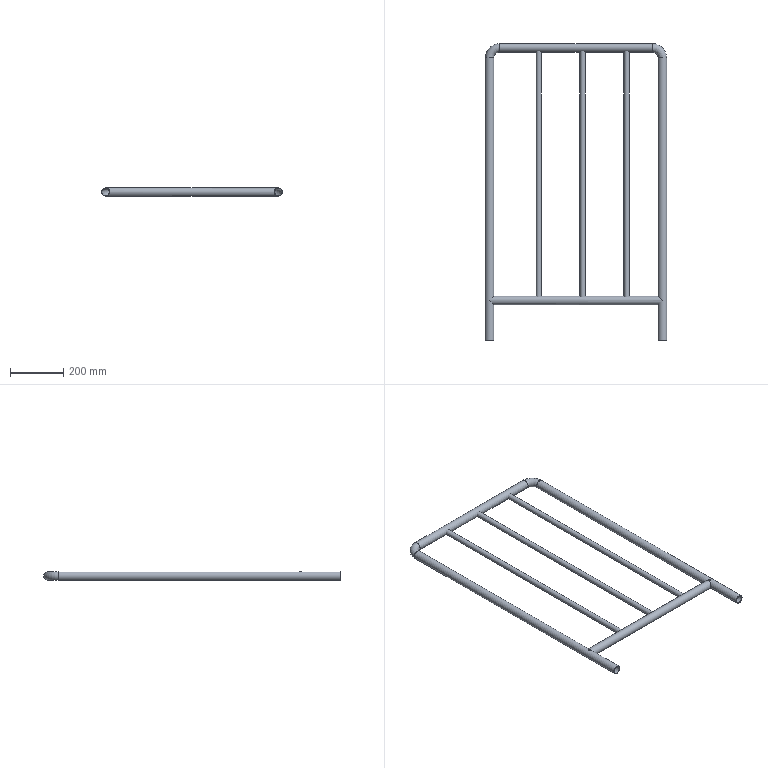Part | STEP file | PN_0011 platform deck 304 guardrail 650X1100_Default<As Machined> | 9 solids | 36 faces | box 682 x 1116 x 32 mm | volume 971799 mm3 | cylinder 16 | plane 16 | torus 4 | commonest cylinder face diameters 32 x6 28 x4 16 x3 20 x3